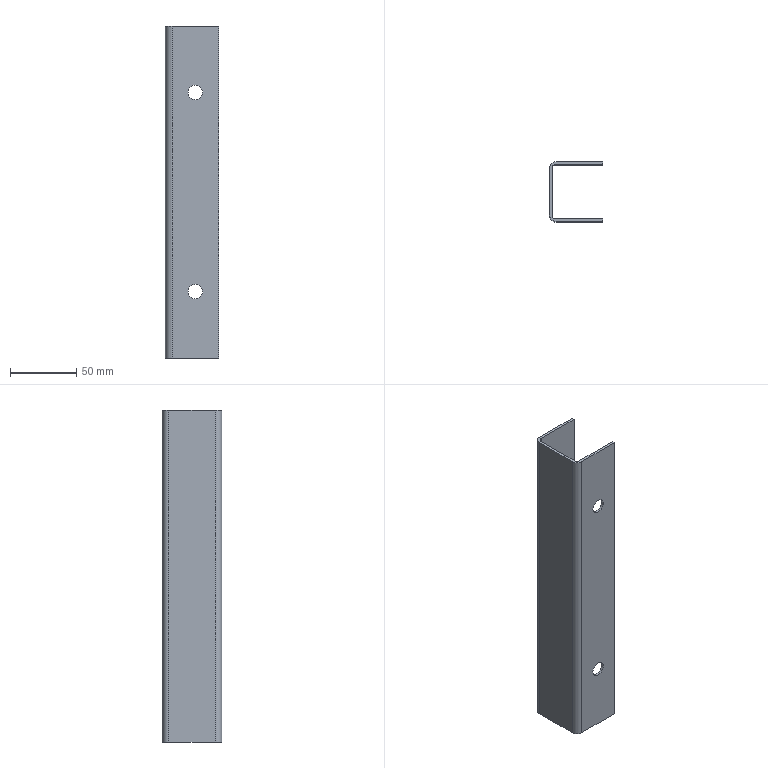Part | STEP file | Channel 50x30x2x3-250 GOST 8278-83 | 1 solid | 18 faces | box 40 x 45 x 250 mm | volume 58023 mm3 | plane 10 | cylinder 8 | commonest cylinder face diameters 11 x4 6 x2 10 x2
STEP:
#1=CARTESIAN_POINT('',(0.,0.,0.));
#2=DIRECTION('',(0.,0.,1.));
#3=DIRECTION('',(1.,0.,0.));
#4=AXIS2_PLACEMENT_3D('',#1,#2,#3);
#5=CARTESIAN_POINT('',(18.8,-18.,200.));
#6=VERTEX_POINT('',#5);
#7=CARTESIAN_POINT('',(13.3,-18.,200.));
#8=DIRECTION('',(0.,-1.,0.));
#9=DIRECTION('',(-1.,0.,0.));
#10=AXIS2_PLACEMENT_3D('',#7,#8,#9);
#11=CIRCLE('',#10,5.5);
#12=CARTESIAN_POINT('',(13.3,25.,200.));
#13=DIRECTION('',(0.,1.,0.));
#14=DIRECTION('',(-1.,0.,0.));
#15=AXIS2_PLACEMENT_3D('',#12,#13,#14);
#16=CYLINDRICAL_SURFACE('',#15,5.5);
#17=CARTESIAN_POINT('',(12.566,-43.));
#18=DIRECTION('',(-1.,0.));
#19=VECTOR('',#18,1.);
#20=LINE('',#17,#19);
#21=(GEOMETRIC_REPRESENTATION_CONTEXT(2)PARAMETRIC_REPRESENTATION_CONTEXT()REPRESENTATION_CONTEXT('',''));
#22=DEFINITIONAL_REPRESENTATION('',(#20),#21);
#23=PCURVE('',#16,#22);
#24=CARTESIAN_POINT('',(-4.2,-18.,0.));
#25=DIRECTION('',(0.,1.,0.));
#26=DIRECTION('',(0.,0.,1.));
#27=AXIS2_PLACEMENT_3D('',#24,#25,#26);
#28=PLANE('',#27);
#29=CARTESIAN_POINT('',(200.,12.));
#30=CARTESIAN_POINT('',(190.474,12.));
#31=CARTESIAN_POINT('',(195.237,20.25));
#32=CARTESIAN_POINT('',(200.,28.5));
#33=CARTESIAN_POINT('',(204.763,20.25));
#34=CARTESIAN_POINT('',(209.526,12.));
#35=CARTESIAN_POINT('',(200.,12.));
#36=(BOUNDED_CURVE()B_SPLINE_CURVE(2,(#29,#30,#31,#32,#33,#34,#35),.UNSPECIFIED.,.T.,.F.)B_SPLINE_CURVE_WITH_KNOTS((1,2,2,2,2,1),(-2.094,0.,2.094,4.189,6.283,8.378),.UNSPECIFIED.)CURVE()GEOMETRIC_REPRESENTATION_ITEM()RATIONAL_B_SPLINE_CURVE((1.,0.5,1.,0.5,1.,0.5,1.))REPRESENTATION_ITEM(''));
#37=(GEOMETRIC_REPRESENTATION_CONTEXT(2)PARAMETRIC_REPRESENTATION_CONTEXT()REPRESENTATION_CONTEXT('',''));
#38=DEFINITIONAL_REPRESENTATION('',(#36),#37);
#39=PCURVE('',#28,#38);
#40=SURFACE_CURVE('',#11,(#23,#39),.PCURVE_S1.);
#41=EDGE_CURVE('',#6,#6,#40,.T.);
#42=ORIENTED_EDGE('',*,*,#41,.T.);
#43=CARTESIAN_POINT('',(18.8,-20.,200.));
#44=VERTEX_POINT('',#43);
#45=CARTESIAN_POINT('',(18.8,-20.,200.));
#46=CARTESIAN_POINT('',(18.8,-18.,200.));
#47=B_SPLINE_CURVE_WITH_KNOTS('',1,(#45,#46),.UNSPECIFIED.,.F.,.F.,(2,2),(-45.,-43.),.PIECEWISE_BEZIER_KNOTS.);
#48=CARTESIAN_POINT('',(3.142,0.));
#49=DIRECTION('',(0.,1.));
#50=VECTOR('',#49,1.);
#51=LINE('',#48,#50);
#52=(GEOMETRIC_REPRESENTATION_CONTEXT(2)PARAMETRIC_REPRESENTATION_CONTEXT()REPRESENTATION_CONTEXT('',''));
#53=DEFINITIONAL_REPRESENTATION('',(#51),#52);
#54=PCURVE('',#16,#53);
#55=CARTESIAN_POINT('',(9.425,0.));
#56=DIRECTION('',(0.,1.));
#57=VECTOR('',#56,1.);
#58=LINE('',#55,#57);
#59=(GEOMETRIC_REPRESENTATION_CONTEXT(2)PARAMETRIC_REPRESENTATION_CONTEXT()REPRESENTATION_CONTEXT('',''));
#60=DEFINITIONAL_REPRESENTATION('',(#58),#59);
#61=PCURVE('',#16,#60);
#62=SEAM_CURVE('',#47,(#54,#61),.PCURVE_S1.);
#63=EDGE_CURVE('',#44,#6,#62,.T.);
#64=ORIENTED_EDGE('',*,*,#63,.F.);
#65=CARTESIAN_POINT('',(13.3,-20.,200.));
#66=DIRECTION('',(0.,1.,0.));
#67=DIRECTION('',(-1.,0.,0.));
#68=AXIS2_PLACEMENT_3D('',#65,#66,#67);
#69=CIRCLE('',#68,5.5);
#70=CARTESIAN_POINT('',(0.,-45.));
#71=DIRECTION('',(1.,0.));
#72=VECTOR('',#71,1.);
#73=LINE('',#70,#72);
#74=(GEOMETRIC_REPRESENTATION_CONTEXT(2)PARAMETRIC_REPRESENTATION_CONTEXT()REPRESENTATION_CONTEXT('',''));
#75=DEFINITIONAL_REPRESENTATION('',(#73),#74);
#76=PCURVE('',#16,#75);
#77=CARTESIAN_POINT('',(30.8,-20.,0.));
#78=DIRECTION('',(0.,-1.,0.));
#79=DIRECTION('',(0.,0.,-1.));
#80=AXIS2_PLACEMENT_3D('',#77,#78,#79);
#81=PLANE('',#80);
#82=CARTESIAN_POINT('',(-200.,-23.));
#83=CARTESIAN_POINT('',(-209.526,-23.));
#84=CARTESIAN_POINT('',(-204.763,-14.75));
#85=CARTESIAN_POINT('',(-200.,-6.5));
#86=CARTESIAN_POINT('',(-195.237,-14.75));
#87=CARTESIAN_POINT('',(-190.474,-23.));
#88=CARTESIAN_POINT('',(-200.,-23.));
#89=(BOUNDED_CURVE()B_SPLINE_CURVE(2,(#82,#83,#84,#85,#86,#87,#88),.UNSPECIFIED.,.T.,.F.)B_SPLINE_CURVE_WITH_KNOTS((1,2,2,2,2,1),(-2.094,0.,2.094,4.189,6.283,8.378),.UNSPECIFIED.)CURVE()GEOMETRIC_REPRESENTATION_ITEM()RATIONAL_B_SPLINE_CURVE((1.,0.5,1.,0.5,1.,0.5,1.))REPRESENTATION_ITEM(''));
#90=(GEOMETRIC_REPRESENTATION_CONTEXT(2)PARAMETRIC_REPRESENTATION_CONTEXT()REPRESENTATION_CONTEXT('',''));
#91=DEFINITIONAL_REPRESENTATION('',(#89),#90);
#92=PCURVE('',#81,#91);
#93=SURFACE_CURVE('',#69,(#76,#92),.PCURVE_S1.);
#94=EDGE_CURVE('',#44,#44,#93,.T.);
#95=ORIENTED_EDGE('',*,*,#94,.T.);
#96=ORIENTED_EDGE('',*,*,#63,.T.);
#97=EDGE_LOOP('',(#42,#64,#95,#96));
#98=FACE_BOUND('',#97,.F.);
#99=ADVANCED_FACE('',(#98),#16,.F.);
#100=CARTESIAN_POINT('',(18.8,25.,200.));
#101=VERTEX_POINT('',#100);
#102=CARTESIAN_POINT('',(13.3,25.,200.));
#103=DIRECTION('',(0.,-1.,0.));
#104=DIRECTION('',(-1.,0.,0.));
#105=AXIS2_PLACEMENT_3D('',#102,#103,#104);
#106=CIRCLE('',#105,5.5);
#107=CARTESIAN_POINT('',(13.3,25.,200.));
#108=DIRECTION('',(0.,1.,0.));
#109=DIRECTION('',(-1.,0.,0.));
#110=AXIS2_PLACEMENT_3D('',#107,#108,#109);
#111=CYLINDRICAL_SURFACE('',#110,5.5);
#112=CARTESIAN_POINT('',(12.566,0.));
#113=DIRECTION('',(-1.,0.));
#114=VECTOR('',#113,1.);
#115=LINE('',#112,#114);
#116=(GEOMETRIC_REPRESENTATION_CONTEXT(2)PARAMETRIC_REPRESENTATION_CONTEXT()REPRESENTATION_CONTEXT('',''));
#117=DEFINITIONAL_REPRESENTATION('',(#115),#116);
#118=PCURVE('',#111,#117);
#119=CARTESIAN_POINT('',(-4.2,25.,0.));
#120=DIRECTION('',(0.,1.,0.));
#121=DIRECTION('',(0.,0.,1.));
#122=AXIS2_PLACEMENT_3D('',#119,#120,#121);
#123=PLANE('',#122);
#124=CARTESIAN_POINT('',(200.,12.));
#125=CARTESIAN_POINT('',(190.474,12.));
#126=CARTESIAN_POINT('',(195.237,20.25));
#127=CARTESIAN_POINT('',(200.,28.5));
#128=CARTESIAN_POINT('',(204.763,20.25));
#129=CARTESIAN_POINT('',(209.526,12.));
#130=CARTESIAN_POINT('',(200.,12.));
#131=(BOUNDED_CURVE()B_SPLINE_CURVE(2,(#124,#125,#126,#127,#128,#129,#130),.UNSPECIFIED.,.T.,.F.)B_SPLINE_CURVE_WITH_KNOTS((1,2,2,2,2,1),(-2.094,0.,2.094,4.189,6.283,8.378),.UNSPECIFIED.)CURVE()GEOMETRIC_REPRESENTATION_ITEM()RATIONAL_B_SPLINE_CURVE((1.,0.5,1.,0.5,1.,0.5,1.))REPRESENTATION_ITEM(''));
#132=(GEOMETRIC_REPRESENTATION_CONTEXT(2)PARAMETRIC_REPRESENTATION_CONTEXT()REPRESENTATION_CONTEXT('',''));
#133=DEFINITIONAL_REPRESENTATION('',(#131),#132);
#134=PCURVE('',#123,#133);
#135=SURFACE_CURVE('',#106,(#118,#134),.PCURVE_S1.);
#136=EDGE_CURVE('',#101,#101,#135,.T.);
#137=ORIENTED_EDGE('',*,*,#136,.T.);
#138=CARTESIAN_POINT('',(18.8,23.,200.));
#139=VERTEX_POINT('',#138);
#140=CARTESIAN_POINT('',(18.8,23.,200.));
#141=CARTESIAN_POINT('',(18.8,25.,200.));
#142=B_SPLINE_CURVE_WITH_KNOTS('',1,(#140,#141),.UNSPECIFIED.,.F.,.F.,(2,2),(-2.,0.),.PIECEWISE_BEZIER_KNOTS.);
#143=CARTESIAN_POINT('',(3.142,0.));
#144=DIRECTION('',(0.,1.));
#145=VECTOR('',#144,1.);
#146=LINE('',#143,#145);
#147=(GEOMETRIC_REPRESENTATION_CONTEXT(2)PARAMETRIC_REPRESENTATION_CONTEXT()REPRESENTATION_CONTEXT('',''));
#148=DEFINITIONAL_REPRESENTATION('',(#146),#147);
#149=PCURVE('',#111,#148);
#150=CARTESIAN_POINT('',(9.425,0.));
#151=DIRECTION('',(0.,1.));
#152=VECTOR('',#151,1.);
#153=LINE('',#150,#152);
#154=(GEOMETRIC_REPRESENTATION_CONTEXT(2)PARAMETRIC_REPRESENTATION_CONTEXT()REPRESENTATION_CONTEXT('',''));
#155=DEFINITIONAL_REPRESENTATION('',(#153),#154);
#156=PCURVE('',#111,#155);
#157=SEAM_CURVE('',#142,(#149,#156),.PCURVE_S1.);
#158=EDGE_CURVE('',#139,#101,#157,.T.);
#159=ORIENTED_EDGE('',*,*,#158,.F.);
#160=CARTESIAN_POINT('',(13.3,23.,200.));
#161=DIRECTION('',(0.,1.,0.));
#162=DIRECTION('',(-1.,0.,0.));
#163=AXIS2_PLACEMENT_3D('',#160,#161,#162);
#164=CIRCLE('',#163,5.5);
#165=CARTESIAN_POINT('',(0.,-2.));
#166=DIRECTION('',(1.,0.));
#167=VECTOR('',#166,1.);
#168=LINE('',#165,#167);
#169=(GEOMETRIC_REPRESENTATION_CONTEXT(2)PARAMETRIC_REPRESENTATION_CONTEXT()REPRESENTATION_CONTEXT('',''));
#170=DEFINITIONAL_REPRESENTATION('',(#168),#169);
#171=PCURVE('',#111,#170);
#172=CARTESIAN_POINT('',(30.8,23.,0.));
#173=DIRECTION('',(0.,-1.,0.));
#174=DIRECTION('',(0.,0.,-1.));
#175=AXIS2_PLACEMENT_3D('',#172,#173,#174);
#176=PLANE('',#175);
#177=CARTESIAN_POINT('',(-200.,-23.));
#178=CARTESIAN_POINT('',(-209.526,-23.));
#179=CARTESIAN_POINT('',(-204.763,-14.75));
#180=CARTESIAN_POINT('',(-200.,-6.5));
#181=CARTESIAN_POINT('',(-195.237,-14.75));
#182=CARTESIAN_POINT('',(-190.474,-23.));
#183=CARTESIAN_POINT('',(-200.,-23.));
#184=(BOUNDED_CURVE()B_SPLINE_CURVE(2,(#177,#178,#179,#180,#181,#182,#183),.UNSPECIFIED.,.T.,.F.)B_SPLINE_CURVE_WITH_KNOTS((1,2,2,2,2,1),(-2.094,0.,2.094,4.189,6.283,8.378),.UNSPECIFIED.)CURVE()GEOMETRIC_REPRESENTATION_ITEM()RATIONAL_B_SPLINE_CURVE((1.,0.5,1.,0.5,1.,0.5,1.))REPRESENTATION_ITEM(''));
#185=(GEOMETRIC_REPRESENTATION_CONTEXT(2)PARAMETRIC_REPRESENTATION_CONTEXT()REPRESENTATION_CONTEXT('',''));
#186=DEFINITIONAL_REPRESENTATION('',(#184),#185);
#187=PCURVE('',#176,#186);
#188=SURFACE_CURVE('',#164,(#171,#187),.PCURVE_S1.);
#189=EDGE_CURVE('',#139,#139,#188,.T.);
#190=ORIENTED_EDGE('',*,*,#189,.T.);
#191=ORIENTED_EDGE('',*,*,#158,.T.);
#192=EDGE_LOOP('',(#137,#159,#190,#191));
#193=FACE_BOUND('',#192,.F.);
#194=ADVANCED_FACE('',(#193),#111,.F.);
#195=CARTESIAN_POINT('',(18.8,-18.,50.));
#196=VERTEX_POINT('',#195);
#197=CARTESIAN_POINT('',(13.3,-18.,50.));
#198=DIRECTION('',(0.,-1.,0.));
#199=DIRECTION('',(-1.,0.,0.));
#200=AXIS2_PLACEMENT_3D('',#197,#198,#199);
#201=CIRCLE('',#200,5.5);
#202=CARTESIAN_POINT('',(13.3,25.,50.));
#203=DIRECTION('',(0.,1.,0.));
#204=DIRECTION('',(-1.,0.,0.));
#205=AXIS2_PLACEMENT_3D('',#202,#203,#204);
#206=CYLINDRICAL_SURFACE('',#205,5.5);
#207=CARTESIAN_POINT('',(12.566,-43.));
#208=DIRECTION('',(-1.,0.));
#209=VECTOR('',#208,1.);
#210=LINE('',#207,#209);
#211=(GEOMETRIC_REPRESENTATION_CONTEXT(2)PARAMETRIC_REPRESENTATION_CONTEXT()REPRESENTATION_CONTEXT('',''));
#212=DEFINITIONAL_REPRESENTATION('',(#210),#211);
#213=PCURVE('',#206,#212);
#214=CARTESIAN_POINT('',(50.,12.));
#215=CARTESIAN_POINT('',(40.474,12.));
#216=CARTESIAN_POINT('',(45.237,20.25));
#217=CARTESIAN_POINT('',(50.,28.5));
#218=CARTESIAN_POINT('',(54.763,20.25));
#219=CARTESIAN_POINT('',(59.526,12.));
#220=CARTESIAN_POINT('',(50.,12.));
#221=(BOUNDED_CURVE()B_SPLINE_CURVE(2,(#214,#215,#216,#217,#218,#219,#220),.UNSPECIFIED.,.T.,.F.)B_SPLINE_CURVE_WITH_KNOTS((1,2,2,2,2,1),(-2.094,0.,2.094,4.189,6.283,8.378),.UNSPECIFIED.)CURVE()GEOMETRIC_REPRESENTATION_ITEM()RATIONAL_B_SPLINE_CURVE((1.,0.5,1.,0.5,1.,0.5,1.))REPRESENTATION_ITEM(''));
#222=(GEOMETRIC_REPRESENTATION_CONTEXT(2)PARAMETRIC_REPRESENTATION_CONTEXT()REPRESENTATION_CONTEXT('',''));
#223=DEFINITIONAL_REPRESENTATION('',(#221),#222);
#224=PCURVE('',#28,#223);
#225=SURFACE_CURVE('',#201,(#213,#224),.PCURVE_S1.);
#226=EDGE_CURVE('',#196,#196,#225,.T.);
#227=ORIENTED_EDGE('',*,*,#226,.T.);
#228=CARTESIAN_POINT('',(18.8,-20.,50.));
#229=VERTEX_POINT('',#228);
#230=CARTESIAN_POINT('',(18.8,-20.,50.));
#231=CARTESIAN_POINT('',(18.8,-18.,50.));
#232=B_SPLINE_CURVE_WITH_KNOTS('',1,(#230,#231),.UNSPECIFIED.,.F.,.F.,(2,2),(-45.,-43.),.PIECEWISE_BEZIER_KNOTS.);
#233=CARTESIAN_POINT('',(3.142,0.));
#234=DIRECTION('',(0.,1.));
#235=VECTOR('',#234,1.);
#236=LINE('',#233,#235);
#237=(GEOMETRIC_REPRESENTATION_CONTEXT(2)PARAMETRIC_REPRESENTATION_CONTEXT()REPRESENTATION_CONTEXT('',''));
#238=DEFINITIONAL_REPRESENTATION('',(#236),#237);
#239=PCURVE('',#206,#238);
#240=CARTESIAN_POINT('',(9.425,0.));
#241=DIRECTION('',(0.,1.));
#242=VECTOR('',#241,1.);
#243=LINE('',#240,#242);
#244=(GEOMETRIC_REPRESENTATION_CONTEXT(2)PARAMETRIC_REPRESENTATION_CONTEXT()REPRESENTATION_CONTEXT('',''));
#245=DEFINITIONAL_REPRESENTATION('',(#243),#244);
#246=PCURVE('',#206,#245);
#247=SEAM_CURVE('',#232,(#239,#246),.PCURVE_S1.);
#248=EDGE_CURVE('',#229,#196,#247,.T.);
#249=ORIENTED_EDGE('',*,*,#248,.F.);
#250=CARTESIAN_POINT('',(13.3,-20.,50.));
#251=DIRECTION('',(0.,1.,0.));
#252=DIRECTION('',(-1.,0.,0.));
#253=AXIS2_PLACEMENT_3D('',#250,#251,#252);
#254=CIRCLE('',#253,5.5);
#255=CARTESIAN_POINT('',(0.,-45.));
#256=DIRECTION('',(1.,0.));
#257=VECTOR('',#256,1.);
#258=LINE('',#255,#257);
#259=(GEOMETRIC_REPRESENTATION_CONTEXT(2)PARAMETRIC_REPRESENTATION_CONTEXT()REPRESENTATION_CONTEXT('',''));
#260=DEFINITIONAL_REPRESENTATION('',(#258),#259);
#261=PCURVE('',#206,#260);
#262=CARTESIAN_POINT('',(-50.,-23.));
#263=CARTESIAN_POINT('',(-59.526,-23.));
#264=CARTESIAN_POINT('',(-54.763,-14.75));
#265=CARTESIAN_POINT('',(-50.,-6.5));
#266=CARTESIAN_POINT('',(-45.237,-14.75));
#267=CARTESIAN_POINT('',(-40.474,-23.));
#268=CARTESIAN_POINT('',(-50.,-23.));
#269=(BOUNDED_CURVE()B_SPLINE_CURVE(2,(#262,#263,#264,#265,#266,#267,#268),.UNSPECIFIED.,.T.,.F.)B_SPLINE_CURVE_WITH_KNOTS((1,2,2,2,2,1),(-2.094,0.,2.094,4.189,6.283,8.378),.UNSPECIFIED.)CURVE()GEOMETRIC_REPRESENTATION_ITEM()RATIONAL_B_SPLINE_CURVE((1.,0.5,1.,0.5,1.,0.5,1.))REPRESENTATION_ITEM(''));
#270=(GEOMETRIC_REPRESENTATION_CONTEXT(2)PARAMETRIC_REPRESENTATION_CONTEXT()REPRESENTATION_CONTEXT('',''));
#271=DEFINITIONAL_REPRESENTATION('',(#269),#270);
#272=PCURVE('',#81,#271);
#273=SURFACE_CURVE('',#254,(#261,#272),.PCURVE_S1.);
#274=EDGE_CURVE('',#229,#229,#273,.T.);
#275=ORIENTED_EDGE('',*,*,#274,.T.);
#276=ORIENTED_EDGE('',*,*,#248,.T.);
#277=EDGE_LOOP('',(#227,#249,#275,#276));
#278=FACE_BOUND('',#277,.F.);
#279=ADVANCED_FACE('',(#278),#206,.F.);
#280=CARTESIAN_POINT('',(18.8,25.,50.));
#281=VERTEX_POINT('',#280);
#282=CARTESIAN_POINT('',(13.3,25.,50.));
#283=DIRECTION('',(0.,-1.,0.));
#284=DIRECTION('',(-1.,0.,0.));
#285=AXIS2_PLACEMENT_3D('',#282,#283,#284);
#286=CIRCLE('',#285,5.5);
#287=CARTESIAN_POINT('',(13.3,25.,50.));
#288=DIRECTION('',(0.,1.,0.));
#289=DIRECTION('',(-1.,0.,0.));
#290=AXIS2_PLACEMENT_3D('',#287,#288,#289);
#291=CYLINDRICAL_SURFACE('',#290,5.5);
#292=CARTESIAN_POINT('',(12.566,0.));
#293=DIRECTION('',(-1.,0.));
#294=VECTOR('',#293,1.);
#295=LINE('',#292,#294);
#296=(GEOMETRIC_REPRESENTATION_CONTEXT(2)PARAMETRIC_REPRESENTATION_CONTEXT()REPRESENTATION_CONTEXT('',''));
#297=DEFINITIONAL_REPRESENTATION('',(#295),#296);
#298=PCURVE('',#291,#297);
#299=CARTESIAN_POINT('',(50.,12.));
#300=CARTESIAN_POINT('',(40.474,12.));
#301=CARTESIAN_POINT('',(45.237,20.25));
#302=CARTESIAN_POINT('',(50.,28.5));
#303=CARTESIAN_POINT('',(54.763,20.25));
#304=CARTESIAN_POINT('',(59.526,12.));
#305=CARTESIAN_POINT('',(50.,12.));
#306=(BOUNDED_CURVE()B_SPLINE_CURVE(2,(#299,#300,#301,#302,#303,#304,#305),.UNSPECIFIED.,.T.,.F.)B_SPLINE_CURVE_WITH_KNOTS((1,2,2,2,2,1),(-2.094,0.,2.094,4.189,6.283,8.378),.UNSPECIFIED.)CURVE()GEOMETRIC_REPRESENTATION_ITEM()RATIONAL_B_SPLINE_CURVE((1.,0.5,1.,0.5,1.,0.5,1.))REPRESENTATION_ITEM(''));
#307=(GEOMETRIC_REPRESENTATION_CONTEXT(2)PARAMETRIC_REPRESENTATION_CONTEXT()REPRESENTATION_CONTEXT('',''));
#308=DEFINITIONAL_REPRESENTATION('',(#306),#307);
#309=PCURVE('',#123,#308);
#310=SURFACE_CURVE('',#286,(#298,#309),.PCURVE_S1.);
#311=EDGE_CURVE('',#281,#281,#310,.T.);
#312=ORIENTED_EDGE('',*,*,#311,.T.);
#313=CARTESIAN_POINT('',(18.8,23.,50.));
#314=VERTEX_POINT('',#313);
#315=CARTESIAN_POINT('',(18.8,23.,50.));
#316=CARTESIAN_POINT('',(18.8,25.,50.));
#317=B_SPLINE_CURVE_WITH_KNOTS('',1,(#315,#316),.UNSPECIFIED.,.F.,.F.,(2,2),(-2.,0.),.PIECEWISE_BEZIER_KNOTS.);
#318=CARTESIAN_POINT('',(3.142,0.));
#319=DIRECTION('',(0.,1.));
#320=VECTOR('',#319,1.);
#321=LINE('',#318,#320);
#322=(GEOMETRIC_REPRESENTATION_CONTEXT(2)PARAMETRIC_REPRESENTATION_CONTEXT()REPRESENTATION_CONTEXT('',''));
#323=DEFINITIONAL_REPRESENTATION('',(#321),#322);
#324=PCURVE('',#291,#323);
#325=CARTESIAN_POINT('',(9.425,0.));
#326=DIRECTION('',(0.,1.));
#327=VECTOR('',#326,1.);
#328=LINE('',#325,#327);
#329=(GEOMETRIC_REPRESENTATION_CONTEXT(2)PARAMETRIC_REPRESENTATION_CONTEXT()REPRESENTATION_CONTEXT('',''));
#330=DEFINITIONAL_REPRESENTATION('',(#328),#329);
#331=PCURVE('',#291,#330);
#332=SEAM_CURVE('',#317,(#324,#331),.PCURVE_S1.);
#333=EDGE_CURVE('',#314,#281,#332,.T.);
#334=ORIENTED_EDGE('',*,*,#333,.F.);
#335=CARTESIAN_POINT('',(13.3,23.,50.));
#336=DIRECTION('',(0.,1.,0.));
#337=DIRECTION('',(-1.,0.,0.));
#338=AXIS2_PLACEMENT_3D('',#335,#336,#337);
#339=CIRCLE('',#338,5.5);
#340=CARTESIAN_POINT('',(0.,-2.));
#341=DIRECTION('',(1.,0.));
#342=VECTOR('',#341,1.);
#343=LINE('',#340,#342);
#344=(GEOMETRIC_REPRESENTATION_CONTEXT(2)PARAMETRIC_REPRESENTATION_CONTEXT()REPRESENTATION_CONTEXT('',''));
#345=DEFINITIONAL_REPRESENTATION('',(#343),#344);
#346=PCURVE('',#291,#345);
#347=CARTESIAN_POINT('',(-50.,-23.));
#348=CARTESIAN_POINT('',(-59.526,-23.));
#349=CARTESIAN_POINT('',(-54.763,-14.75));
#350=CARTESIAN_POINT('',(-50.,-6.5));
#351=CARTESIAN_POINT('',(-45.237,-14.75));
#352=CARTESIAN_POINT('',(-40.474,-23.));
#353=CARTESIAN_POINT('',(-50.,-23.));
#354=(BOUNDED_CURVE()B_SPLINE_CURVE(2,(#347,#348,#349,#350,#351,#352,#353),.UNSPECIFIED.,.T.,.F.)B_SPLINE_CURVE_WITH_KNOTS((1,2,2,2,2,1),(-2.094,0.,2.094,4.189,6.283,8.378),.UNSPECIFIED.)CURVE()GEOMETRIC_REPRESENTATION_ITEM()RATIONAL_B_SPLINE_CURVE((1.,0.5,1.,0.5,1.,0.5,1.))REPRESENTATION_ITEM(''));
#355=(GEOMETRIC_REPRESENTATION_CONTEXT(2)PARAMETRIC_REPRESENTATION_CONTEXT()REPRESENTATION_CONTEXT('',''));
#356=DEFINITIONAL_REPRESENTATION('',(#354),#355);
#357=PCURVE('',#176,#356);
#358=SURFACE_CURVE('',#339,(#346,#357),.PCURVE_S1.);
#359=EDGE_CURVE('',#314,#314,#358,.T.);
#360=ORIENTED_EDGE('',*,*,#359,.T.);
#361=ORIENTED_EDGE('',*,*,#333,.T.);
#362=EDGE_LOOP('',(#312,#334,#360,#361));
#363=FACE_BOUND('',#362,.F.);
#364=ADVANCED_FACE('',(#363),#291,.F.);
#365=CARTESIAN_POINT('',(30.8,-20.,250.));
#366=VERTEX_POINT('',#365);
#367=CARTESIAN_POINT('',(-4.2,-20.,250.));
#368=VERTEX_POINT('',#367);
#369=CARTESIAN_POINT('',(20.8,-20.,250.));
#370=DIRECTION('',(-1.,0.,0.));
#371=VECTOR('',#370,1.);
#372=LINE('',#369,#371);
#373=CARTESIAN_POINT('',(-250.,-10.));
#374=DIRECTION('',(0.,-1.));
#375=VECTOR('',#374,1.);
#376=LINE('',#373,#375);
#377=(GEOMETRIC_REPRESENTATION_CONTEXT(2)PARAMETRIC_REPRESENTATION_CONTEXT()REPRESENTATION_CONTEXT('',''));
#378=DEFINITIONAL_REPRESENTATION('',(#376),#377);
#379=PCURVE('',#81,#378);
#380=CARTESIAN_POINT('',(10.8,2.5,250.));
#381=DIRECTION('',(0.,0.,1.));
#382=DIRECTION('',(1.,0.,0.));
#383=AXIS2_PLACEMENT_3D('',#380,#381,#382);
#384=PLANE('',#383);
#385=CARTESIAN_POINT('',(10.,-22.5));
#386=DIRECTION('',(-1.,0.));
#387=VECTOR('',#386,1.);
#388=LINE('',#385,#387);
#389=(GEOMETRIC_REPRESENTATION_CONTEXT(2)PARAMETRIC_REPRESENTATION_CONTEXT()REPRESENTATION_CONTEXT('',''));
#390=DEFINITIONAL_REPRESENTATION('',(#388),#389);
#391=PCURVE('',#384,#390);
#392=SURFACE_CURVE('',#372,(#379,#391),.PCURVE_S1.);
#393=EDGE_CURVE('',#366,#368,#392,.T.);
#394=ORIENTED_EDGE('',*,*,#393,.T.);
#395=CARTESIAN_POINT('',(-4.2,-20.,0.));
#396=VERTEX_POINT('',#395);
#397=CARTESIAN_POINT('',(-4.2,-20.,0.));
#398=DIRECTION('',(0.,0.,1.));
#399=VECTOR('',#398,1.);
#400=LINE('',#397,#399);
#401=CARTESIAN_POINT('',(0.,-35.));
#402=DIRECTION('',(-1.,0.));
#403=VECTOR('',#402,1.);
#404=LINE('',#401,#403);
#405=(GEOMETRIC_REPRESENTATION_CONTEXT(2)PARAMETRIC_REPRESENTATION_CONTEXT()REPRESENTATION_CONTEXT('',''));
#406=DEFINITIONAL_REPRESENTATION('',(#404),#405);
#407=PCURVE('',#81,#406);
#408=CARTESIAN_POINT('',(-4.2,-15.,0.));
#409=DIRECTION('',(0.,0.,1.));
#410=DIRECTION('',(1.,0.,0.));
#411=AXIS2_PLACEMENT_3D('',#408,#409,#410);
#412=CYLINDRICAL_SURFACE('',#411,5.);
#413=CARTESIAN_POINT('',(4.712,0.));
#414=DIRECTION('',(0.,1.));
#415=VECTOR('',#414,1.);
#416=LINE('',#413,#415);
#417=(GEOMETRIC_REPRESENTATION_CONTEXT(2)PARAMETRIC_REPRESENTATION_CONTEXT()REPRESENTATION_CONTEXT('',''));
#418=DEFINITIONAL_REPRESENTATION('',(#416),#417);
#419=PCURVE('',#412,#418);
#420=SURFACE_CURVE('',#400,(#407,#419),.PCURVE_S1.);
#421=EDGE_CURVE('',#396,#368,#420,.T.);
#422=ORIENTED_EDGE('',*,*,#421,.F.);
#423=CARTESIAN_POINT('',(30.8,-20.,0.));
#424=VERTEX_POINT('',#423);
#425=CARTESIAN_POINT('',(20.8,-20.,0.));
#426=DIRECTION('',(-1.,0.,0.));
#427=VECTOR('',#426,1.);
#428=LINE('',#425,#427);
#429=CARTESIAN_POINT('',(0.,-10.));
#430=DIRECTION('',(0.,-1.));
#431=VECTOR('',#430,1.);
#432=LINE('',#429,#431);
#433=(GEOMETRIC_REPRESENTATION_CONTEXT(2)PARAMETRIC_REPRESENTATION_CONTEXT()REPRESENTATION_CONTEXT('',''));
#434=DEFINITIONAL_REPRESENTATION('',(#432),#433);
#435=PCURVE('',#81,#434);
#436=CARTESIAN_POINT('',(10.8,2.5,0.));
#437=DIRECTION('',(0.,0.,1.));
#438=DIRECTION('',(1.,0.,0.));
#439=AXIS2_PLACEMENT_3D('',#436,#437,#438);
#440=PLANE('',#439);
#441=CARTESIAN_POINT('',(10.,-22.5));
#442=DIRECTION('',(-1.,0.));
#443=VECTOR('',#442,1.);
#444=LINE('',#441,#443);
#445=(GEOMETRIC_REPRESENTATION_CONTEXT(2)PARAMETRIC_REPRESENTATION_CONTEXT()REPRESENTATION_CONTEXT('',''));
#446=DEFINITIONAL_REPRESENTATION('',(#444),#445);
#447=PCURVE('',#440,#446);
#448=SURFACE_CURVE('',#428,(#435,#447),.PCURVE_S1.);
#449=EDGE_CURVE('',#424,#396,#448,.T.);
#450=ORIENTED_EDGE('',*,*,#449,.F.);
#451=CARTESIAN_POINT('',(30.8,-20.,0.));
#452=DIRECTION('',(0.,0.,1.));
#453=VECTOR('',#452,1.);
#454=LINE('',#451,#453);
#455=CARTESIAN_POINT('',(0.,0.));
#456=DIRECTION('',(-1.,0.));
#457=VECTOR('',#456,1.);
#458=LINE('',#455,#457);
#459=(GEOMETRIC_REPRESENTATION_CONTEXT(2)PARAMETRIC_REPRESENTATION_CONTEXT()REPRESENTATION_CONTEXT('',''));
#460=DEFINITIONAL_REPRESENTATION('',(#458),#459);
#461=PCURVE('',#81,#460);
#462=CARTESIAN_POINT('',(30.8,-18.,0.));
#463=DIRECTION('',(1.,0.,0.));
#464=DIRECTION('',(0.,0.,-1.));
#465=AXIS2_PLACEMENT_3D('',#462,#463,#464);
#466=PLANE('',#465);
#467=CARTESIAN_POINT('',(0.,-2.));
#468=DIRECTION('',(-1.,0.));
#469=VECTOR('',#468,1.);
#470=LINE('',#467,#469);
#471=(GEOMETRIC_REPRESENTATION_CONTEXT(2)PARAMETRIC_REPRESENTATION_CONTEXT()REPRESENTATION_CONTEXT('',''));
#472=DEFINITIONAL_REPRESENTATION('',(#470),#471);
#473=PCURVE('',#466,#472);
#474=SURFACE_CURVE('',#454,(#461,#473),.PCURVE_S1.);
#475=EDGE_CURVE('',#424,#366,#474,.T.);
#476=ORIENTED_EDGE('',*,*,#475,.T.);
#477=EDGE_LOOP('',(#394,#422,#450,#476));
#478=FACE_BOUND('',#477,.T.);
#479=ORIENTED_EDGE('',*,*,#94,.T.);
#480=EDGE_LOOP('',(#479));
#481=FACE_BOUND('',#480,.T.);
#482=ORIENTED_EDGE('',*,*,#274,.T.);
#483=EDGE_LOOP('',(#482));
#484=FACE_BOUND('',#483,.T.);
#485=ADVANCED_FACE('',(#478,#481,#484),#81,.T.);
#486=CARTESIAN_POINT('',(-9.2,-15.,250.));
#487=VERTEX_POINT('',#486);
#488=CARTESIAN_POINT('',(-4.2,-15.,250.));
#489=DIRECTION('',(0.,0.,-1.));
#490=DIRECTION('',(1.,0.,0.));
#491=AXIS2_PLACEMENT_3D('',#488,#489,#490);
#492=CIRCLE('',#491,5.);
#493=CARTESIAN_POINT('',(6.283,250.));
#494=DIRECTION('',(-1.,0.));
#495=VECTOR('',#494,1.);
#496=LINE('',#493,#495);
#497=(GEOMETRIC_REPRESENTATION_CONTEXT(2)PARAMETRIC_REPRESENTATION_CONTEXT()REPRESENTATION_CONTEXT('',''));
#498=DEFINITIONAL_REPRESENTATION('',(#496),#497);
#499=PCURVE('',#412,#498);
#500=CARTESIAN_POINT('',(-10.,-17.5));
#501=CARTESIAN_POINT('',(-10.,-26.16));
#502=CARTESIAN_POINT('',(-17.5,-21.83));
#503=CARTESIAN_POINT('',(-25.,-17.5));
#504=CARTESIAN_POINT('',(-17.5,-13.17));
#505=CARTESIAN_POINT('',(-10.,-8.84));
#506=CARTESIAN_POINT('',(-10.,-17.5));
#507=(BOUNDED_CURVE()B_SPLINE_CURVE(2,(#500,#501,#502,#503,#504,#505,#506),.UNSPECIFIED.,.T.,.F.)B_SPLINE_CURVE_WITH_KNOTS((1,2,2,2,2,1),(-2.094,0.,2.094,4.189,6.283,8.378),.UNSPECIFIED.)CURVE()GEOMETRIC_REPRESENTATION_ITEM()RATIONAL_B_SPLINE_CURVE((1.,0.5,1.,0.5,1.,0.5,1.))REPRESENTATION_ITEM(''));
#508=(GEOMETRIC_REPRESENTATION_CONTEXT(2)PARAMETRIC_REPRESENTATION_CONTEXT()REPRESENTATION_CONTEXT('',''));
#509=DEFINITIONAL_REPRESENTATION('',(#507),#508);
#510=PCURVE('',#384,#509);
#511=SURFACE_CURVE('',#492,(#499,#510),.PCURVE_S1.);
#512=EDGE_CURVE('',#368,#487,#511,.T.);
#513=ORIENTED_EDGE('',*,*,#512,.T.);
#514=CARTESIAN_POINT('',(-9.2,-15.,0.));
#515=VERTEX_POINT('',#514);
#516=CARTESIAN_POINT('',(-9.2,-15.,0.));
#517=DIRECTION('',(0.,0.,1.));
#518=VECTOR('',#517,1.);
#519=LINE('',#516,#518);
#520=CARTESIAN_POINT('',(3.142,0.));
#521=DIRECTION('',(0.,1.));
#522=VECTOR('',#521,1.);
#523=LINE('',#520,#522);
#524=(GEOMETRIC_REPRESENTATION_CONTEXT(2)PARAMETRIC_REPRESENTATION_CONTEXT()REPRESENTATION_CONTEXT('',''));
#525=DEFINITIONAL_REPRESENTATION('',(#523),#524);
#526=PCURVE('',#412,#525);
#527=CARTESIAN_POINT('',(-9.2,-15.,0.));
#528=DIRECTION('',(-1.,0.,0.));
#529=DIRECTION('',(0.,0.,1.));
#530=AXIS2_PLACEMENT_3D('',#527,#528,#529);
#531=PLANE('',#530);
#532=CARTESIAN_POINT('',(0.,0.));
#533=DIRECTION('',(1.,0.));
#534=VECTOR('',#533,1.);
#535=LINE('',#532,#534);
#536=(GEOMETRIC_REPRESENTATION_CONTEXT(2)PARAMETRIC_REPRESENTATION_CONTEXT()REPRESENTATION_CONTEXT('',''));
#537=DEFINITIONAL_REPRESENTATION('',(#535),#536);
#538=PCURVE('',#531,#537);
#539=SURFACE_CURVE('',#519,(#526,#538),.PCURVE_S1.);
#540=EDGE_CURVE('',#515,#487,#539,.T.);
#541=ORIENTED_EDGE('',*,*,#540,.F.);
#542=CARTESIAN_POINT('',(-4.2,-15.,0.));
#543=DIRECTION('',(0.,0.,-1.));
#544=DIRECTION('',(1.,0.,0.));
#545=AXIS2_PLACEMENT_3D('',#542,#543,#544);
#546=CIRCLE('',#545,5.);
#547=CARTESIAN_POINT('',(6.283,0.));
#548=DIRECTION('',(-1.,0.));
#549=VECTOR('',#548,1.);
#550=LINE('',#547,#549);
#551=(GEOMETRIC_REPRESENTATION_CONTEXT(2)PARAMETRIC_REPRESENTATION_CONTEXT()REPRESENTATION_CONTEXT('',''));
#552=DEFINITIONAL_REPRESENTATION('',(#550),#551);
#553=PCURVE('',#412,#552);
#554=CARTESIAN_POINT('',(-10.,-17.5));
#555=CARTESIAN_POINT('',(-10.,-26.16));
#556=CARTESIAN_POINT('',(-17.5,-21.83));
#557=CARTESIAN_POINT('',(-25.,-17.5));
#558=CARTESIAN_POINT('',(-17.5,-13.17));
#559=CARTESIAN_POINT('',(-10.,-8.84));
#560=CARTESIAN_POINT('',(-10.,-17.5));
#561=(BOUNDED_CURVE()B_SPLINE_CURVE(2,(#554,#555,#556,#557,#558,#559,#560),.UNSPECIFIED.,.T.,.F.)B_SPLINE_CURVE_WITH_KNOTS((1,2,2,2,2,1),(-2.094,0.,2.094,4.189,6.283,8.378),.UNSPECIFIED.)CURVE()GEOMETRIC_REPRESENTATION_ITEM()RATIONAL_B_SPLINE_CURVE((1.,0.5,1.,0.5,1.,0.5,1.))REPRESENTATION_ITEM(''));
#562=(GEOMETRIC_REPRESENTATION_CONTEXT(2)PARAMETRIC_REPRESENTATION_CONTEXT()REPRESENTATION_CONTEXT('',''));
#563=DEFINITIONAL_REPRESENTATION('',(#561),#562);
#564=PCURVE('',#440,#563);
#565=SURFACE_CURVE('',#546,(#553,#564),.PCURVE_S1.);
#566=EDGE_CURVE('',#396,#515,#565,.T.);
#567=ORIENTED_EDGE('',*,*,#566,.F.);
#568=ORIENTED_EDGE('',*,*,#421,.T.);
#569=EDGE_LOOP('',(#513,#541,#567,#568));
#570=FACE_BOUND('',#569,.T.);
#571=ADVANCED_FACE('',(#570),#412,.T.);
#572=CARTESIAN_POINT('',(-9.2,20.,250.));
#573=VERTEX_POINT('',#572);
#574=CARTESIAN_POINT('',(-9.2,-6.25,250.));
#575=DIRECTION('',(0.,1.,0.));
#576=VECTOR('',#575,1.);
#577=LINE('',#574,#576);
#578=CARTESIAN_POINT('',(250.,8.75));
#579=DIRECTION('',(0.,1.));
#580=VECTOR('',#579,1.);
#581=LINE('',#578,#580);
#582=(GEOMETRIC_REPRESENTATION_CONTEXT(2)PARAMETRIC_REPRESENTATION_CONTEXT()REPRESENTATION_CONTEXT('',''));
#583=DEFINITIONAL_REPRESENTATION('',(#581),#582);
#584=PCURVE('',#531,#583);
#585=CARTESIAN_POINT('',(-20.,-8.75));
#586=DIRECTION('',(0.,1.));
#587=VECTOR('',#586,1.);
#588=LINE('',#585,#587);
#589=(GEOMETRIC_REPRESENTATION_CONTEXT(2)PARAMETRIC_REPRESENTATION_CONTEXT()REPRESENTATION_CONTEXT('',''));
#590=DEFINITIONAL_REPRESENTATION('',(#588),#589);
#591=PCURVE('',#384,#590);
#592=SURFACE_CURVE('',#577,(#584,#591),.PCURVE_S1.);
#593=EDGE_CURVE('',#487,#573,#592,.T.);
#594=ORIENTED_EDGE('',*,*,#593,.T.);
#595=CARTESIAN_POINT('',(-9.2,20.,0.));
#596=VERTEX_POINT('',#595);
#597=CARTESIAN_POINT('',(-9.2,20.,0.));
#598=DIRECTION('',(0.,0.,1.));
#599=VECTOR('',#598,1.);
#600=LINE('',#597,#599);
#601=CARTESIAN_POINT('',(0.,35.));
#602=DIRECTION('',(1.,0.));
#603=VECTOR('',#602,1.);
#604=LINE('',#601,#603);
#605=(GEOMETRIC_REPRESENTATION_CONTEXT(2)PARAMETRIC_REPRESENTATION_CONTEXT()REPRESENTATION_CONTEXT('',''));
#606=DEFINITIONAL_REPRESENTATION('',(#604),#605);
#607=PCURVE('',#531,#606);
#608=CARTESIAN_POINT('',(-4.2,20.,0.));
#609=DIRECTION('',(0.,0.,1.));
#610=DIRECTION('',(0.,-1.,0.));
#611=AXIS2_PLACEMENT_3D('',#608,#609,#610);
#612=CYLINDRICAL_SURFACE('',#611,5.);
#613=CARTESIAN_POINT('',(4.712,0.));
#614=DIRECTION('',(0.,1.));
#615=VECTOR('',#614,1.);
#616=LINE('',#613,#615);
#617=(GEOMETRIC_REPRESENTATION_CONTEXT(2)PARAMETRIC_REPRESENTATION_CONTEXT()REPRESENTATION_CONTEXT('',''));
#618=DEFINITIONAL_REPRESENTATION('',(#616),#617);
#619=PCURVE('',#612,#618);
#620=SURFACE_CURVE('',#600,(#607,#619),.PCURVE_S1.);
#621=EDGE_CURVE('',#596,#573,#620,.T.);
#622=ORIENTED_EDGE('',*,*,#621,.F.);
#623=CARTESIAN_POINT('',(-9.2,-6.25,0.));
#624=DIRECTION('',(0.,1.,0.));
#625=VECTOR('',#624,1.);
#626=LINE('',#623,#625);
#627=CARTESIAN_POINT('',(0.,8.75));
#628=DIRECTION('',(0.,1.));
#629=VECTOR('',#628,1.);
#630=LINE('',#627,#629);
#631=(GEOMETRIC_REPRESENTATION_CONTEXT(2)PARAMETRIC_REPRESENTATION_CONTEXT()REPRESENTATION_CONTEXT('',''));
#632=DEFINITIONAL_REPRESENTATION('',(#630),#631);
#633=PCURVE('',#531,#632);
#634=CARTESIAN_POINT('',(-20.,-8.75));
#635=DIRECTION('',(0.,1.));
#636=VECTOR('',#635,1.);
#637=LINE('',#634,#636);
#638=(GEOMETRIC_REPRESENTATION_CONTEXT(2)PARAMETRIC_REPRESENTATION_CONTEXT()REPRESENTATION_CONTEXT('',''));
#639=DEFINITIONAL_REPRESENTATION('',(#637),#638);
#640=PCURVE('',#440,#639);
#641=SURFACE_CURVE('',#626,(#633,#640),.PCURVE_S1.);
#642=EDGE_CURVE('',#515,#596,#641,.T.);
#643=ORIENTED_EDGE('',*,*,#642,.F.);
#644=ORIENTED_EDGE('',*,*,#540,.T.);
#645=EDGE_LOOP('',(#594,#622,#643,#644));
#646=FACE_BOUND('',#645,.T.);
#647=ADVANCED_FACE('',(#646),#531,.T.);
#648=CARTESIAN_POINT('',(-4.2,25.,250.));
#649=VERTEX_POINT('',#648);
#650=CARTESIAN_POINT('',(-4.2,20.,250.));
#651=DIRECTION('',(0.,0.,-1.));
#652=DIRECTION('',(0.,-1.,0.));
#653=AXIS2_PLACEMENT_3D('',#650,#651,#652);
#654=CIRCLE('',#653,5.);
#655=CARTESIAN_POINT('',(6.283,250.));
#656=DIRECTION('',(-1.,0.));
#657=VECTOR('',#656,1.);
#658=LINE('',#655,#657);
#659=(GEOMETRIC_REPRESENTATION_CONTEXT(2)PARAMETRIC_REPRESENTATION_CONTEXT()REPRESENTATION_CONTEXT('',''));
#660=DEFINITIONAL_REPRESENTATION('',(#658),#659);
#661=PCURVE('',#612,#660);
#662=CARTESIAN_POINT('',(-15.,12.5));
#663=CARTESIAN_POINT('',(-23.66,12.5));
#664=CARTESIAN_POINT('',(-19.33,20.));
#665=CARTESIAN_POINT('',(-15.,27.5));
#666=CARTESIAN_POINT('',(-10.67,20.));
#667=CARTESIAN_POINT('',(-6.34,12.5));
#668=CARTESIAN_POINT('',(-15.,12.5));
#669=(BOUNDED_CURVE()B_SPLINE_CURVE(2,(#662,#663,#664,#665,#666,#667,#668),.UNSPECIFIED.,.T.,.F.)B_SPLINE_CURVE_WITH_KNOTS((1,2,2,2,2,1),(-2.094,0.,2.094,4.189,6.283,8.378),.UNSPECIFIED.)CURVE()GEOMETRIC_REPRESENTATION_ITEM()RATIONAL_B_SPLINE_CURVE((1.,0.5,1.,0.5,1.,0.5,1.))REPRESENTATION_ITEM(''));
#670=(GEOMETRIC_REPRESENTATION_CONTEXT(2)PARAMETRIC_REPRESENTATION_CONTEXT()REPRESENTATION_CONTEXT('',''));
#671=DEFINITIONAL_REPRESENTATION('',(#669),#670);
#672=PCURVE('',#384,#671);
#673=SURFACE_CURVE('',#654,(#661,#672),.PCURVE_S1.);
#674=EDGE_CURVE('',#573,#649,#673,.T.);
#675=ORIENTED_EDGE('',*,*,#674,.T.);
#676=CARTESIAN_POINT('',(-4.2,25.,0.));
#677=VERTEX_POINT('',#676);
#678=CARTESIAN_POINT('',(-4.2,25.,0.));
#679=DIRECTION('',(0.,0.,1.));
#680=VECTOR('',#679,1.);
#681=LINE('',#678,#680);
#682=CARTESIAN_POINT('',(3.142,0.));
#683=DIRECTION('',(0.,1.));
#684=VECTOR('',#683,1.);
#685=LINE('',#682,#684);
#686=(GEOMETRIC_REPRESENTATION_CONTEXT(2)PARAMETRIC_REPRESENTATION_CONTEXT()REPRESENTATION_CONTEXT('',''));
#687=DEFINITIONAL_REPRESENTATION('',(#685),#686);
#688=PCURVE('',#612,#687);
#689=CARTESIAN_POINT('',(0.,0.));
#690=DIRECTION('',(1.,0.));
#691=VECTOR('',#690,1.);
#692=LINE('',#689,#691);
#693=(GEOMETRIC_REPRESENTATION_CONTEXT(2)PARAMETRIC_REPRESENTATION_CONTEXT()REPRESENTATION_CONTEXT('',''));
#694=DEFINITIONAL_REPRESENTATION('',(#692),#693);
#695=PCURVE('',#123,#694);
#696=SURFACE_CURVE('',#681,(#688,#695),.PCURVE_S1.);
#697=EDGE_CURVE('',#677,#649,#696,.T.);
#698=ORIENTED_EDGE('',*,*,#697,.F.);
#699=CARTESIAN_POINT('',(-4.2,20.,0.));
#700=DIRECTION('',(0.,0.,-1.));
#701=DIRECTION('',(0.,-1.,0.));
#702=AXIS2_PLACEMENT_3D('',#699,#700,#701);
#703=CIRCLE('',#702,5.);
#704=CARTESIAN_POINT('',(6.283,0.));
#705=DIRECTION('',(-1.,0.));
#706=VECTOR('',#705,1.);
#707=LINE('',#704,#706);
#708=(GEOMETRIC_REPRESENTATION_CONTEXT(2)PARAMETRIC_REPRESENTATION_CONTEXT()REPRESENTATION_CONTEXT('',''));
#709=DEFINITIONAL_REPRESENTATION('',(#707),#708);
#710=PCURVE('',#612,#709);
#711=CARTESIAN_POINT('',(-15.,12.5));
#712=CARTESIAN_POINT('',(-23.66,12.5));
#713=CARTESIAN_POINT('',(-19.33,20.));
#714=CARTESIAN_POINT('',(-15.,27.5));
#715=CARTESIAN_POINT('',(-10.67,20.));
#716=CARTESIAN_POINT('',(-6.34,12.5));
#717=CARTESIAN_POINT('',(-15.,12.5));
#718=(BOUNDED_CURVE()B_SPLINE_CURVE(2,(#711,#712,#713,#714,#715,#716,#717),.UNSPECIFIED.,.T.,.F.)B_SPLINE_CURVE_WITH_KNOTS((1,2,2,2,2,1),(-2.094,0.,2.094,4.189,6.283,8.378),.UNSPECIFIED.)CURVE()GEOMETRIC_REPRESENTATION_ITEM()RATIONAL_B_SPLINE_CURVE((1.,0.5,1.,0.5,1.,0.5,1.))REPRESENTATION_ITEM(''));
#719=(GEOMETRIC_REPRESENTATION_CONTEXT(2)PARAMETRIC_REPRESENTATION_CONTEXT()REPRESENTATION_CONTEXT('',''));
#720=DEFINITIONAL_REPRESENTATION('',(#718),#719);
#721=PCURVE('',#440,#720);
#722=SURFACE_CURVE('',#703,(#710,#721),.PCURVE_S1.);
#723=EDGE_CURVE('',#596,#677,#722,.T.);
#724=ORIENTED_EDGE('',*,*,#723,.F.);
#725=ORIENTED_EDGE('',*,*,#621,.T.);
#726=EDGE_LOOP('',(#675,#698,#724,#725));
#727=FACE_BOUND('',#726,.T.);
#728=ADVANCED_FACE('',(#727),#612,.T.);
#729=CARTESIAN_POINT('',(30.8,25.,250.));
#730=VERTEX_POINT('',#729);
#731=CARTESIAN_POINT('',(3.3,25.,250.));
#732=DIRECTION('',(1.,0.,0.));
#733=VECTOR('',#732,1.);
#734=LINE('',#731,#733);
#735=CARTESIAN_POINT('',(250.,7.5));
#736=DIRECTION('',(0.,1.));
#737=VECTOR('',#736,1.);
#738=LINE('',#735,#737);
#739=(GEOMETRIC_REPRESENTATION_CONTEXT(2)PARAMETRIC_REPRESENTATION_CONTEXT()REPRESENTATION_CONTEXT('',''));
#740=DEFINITIONAL_REPRESENTATION('',(#738),#739);
#741=PCURVE('',#123,#740);
#742=CARTESIAN_POINT('',(-7.5,22.5));
#743=DIRECTION('',(1.,0.));
#744=VECTOR('',#743,1.);
#745=LINE('',#742,#744);
#746=(GEOMETRIC_REPRESENTATION_CONTEXT(2)PARAMETRIC_REPRESENTATION_CONTEXT()REPRESENTATION_CONTEXT('',''));
#747=DEFINITIONAL_REPRESENTATION('',(#745),#746);
#748=PCURVE('',#384,#747);
#749=SURFACE_CURVE('',#734,(#741,#748),.PCURVE_S1.);
#750=EDGE_CURVE('',#649,#730,#749,.T.);
#751=ORIENTED_EDGE('',*,*,#750,.T.);
#752=CARTESIAN_POINT('',(30.8,25.,0.));
#753=VERTEX_POINT('',#752);
#754=CARTESIAN_POINT('',(30.8,25.,0.));
#755=DIRECTION('',(0.,0.,1.));
#756=VECTOR('',#755,1.);
#757=LINE('',#754,#756);
#758=CARTESIAN_POINT('',(0.,35.));
#759=DIRECTION('',(1.,0.));
#760=VECTOR('',#759,1.);
#761=LINE('',#758,#760);
#762=(GEOMETRIC_REPRESENTATION_CONTEXT(2)PARAMETRIC_REPRESENTATION_CONTEXT()REPRESENTATION_CONTEXT('',''));
#763=DEFINITIONAL_REPRESENTATION('',(#761),#762);
#764=PCURVE('',#123,#763);
#765=CARTESIAN_POINT('',(30.8,25.,0.));
#766=DIRECTION('',(1.,0.,0.));
#767=DIRECTION('',(0.,0.,-1.));
#768=AXIS2_PLACEMENT_3D('',#765,#766,#767);
#769=PLANE('',#768);
#770=CARTESIAN_POINT('',(0.,0.));
#771=DIRECTION('',(-1.,0.));
#772=VECTOR('',#771,1.);
#773=LINE('',#770,#772);
#774=(GEOMETRIC_REPRESENTATION_CONTEXT(2)PARAMETRIC_REPRESENTATION_CONTEXT()REPRESENTATION_CONTEXT('',''));
#775=DEFINITIONAL_REPRESENTATION('',(#773),#774);
#776=PCURVE('',#769,#775);
#777=SURFACE_CURVE('',#757,(#764,#776),.PCURVE_S1.);
#778=EDGE_CURVE('',#753,#730,#777,.T.);
#779=ORIENTED_EDGE('',*,*,#778,.F.);
#780=CARTESIAN_POINT('',(3.3,25.,0.));
#781=DIRECTION('',(1.,0.,0.));
#782=VECTOR('',#781,1.);
#783=LINE('',#780,#782);
#784=CARTESIAN_POINT('',(0.,7.5));
#785=DIRECTION('',(0.,1.));
#786=VECTOR('',#785,1.);
#787=LINE('',#784,#786);
#788=(GEOMETRIC_REPRESENTATION_CONTEXT(2)PARAMETRIC_REPRESENTATION_CONTEXT()REPRESENTATION_CONTEXT('',''));
#789=DEFINITIONAL_REPRESENTATION('',(#787),#788);
#790=PCURVE('',#123,#789);
#791=CARTESIAN_POINT('',(-7.5,22.5));
#792=DIRECTION('',(1.,0.));
#793=VECTOR('',#792,1.);
#794=LINE('',#791,#793);
#795=(GEOMETRIC_REPRESENTATION_CONTEXT(2)PARAMETRIC_REPRESENTATION_CONTEXT()REPRESENTATION_CONTEXT('',''));
#796=DEFINITIONAL_REPRESENTATION('',(#794),#795);
#797=PCURVE('',#440,#796);
#798=SURFACE_CURVE('',#783,(#790,#797),.PCURVE_S1.);
#799=EDGE_CURVE('',#677,#753,#798,.T.);
#800=ORIENTED_EDGE('',*,*,#799,.F.);
#801=ORIENTED_EDGE('',*,*,#697,.T.);
#802=EDGE_LOOP('',(#751,#779,#800,#801));
#803=FACE_BOUND('',#802,.T.);
#804=ORIENTED_EDGE('',*,*,#136,.T.);
#805=EDGE_LOOP('',(#804));
#806=FACE_BOUND('',#805,.T.);
#807=ORIENTED_EDGE('',*,*,#311,.T.);
#808=EDGE_LOOP('',(#807));
#809=FACE_BOUND('',#808,.T.);
#810=ADVANCED_FACE('',(#803,#806,#809),#123,.T.);
#811=CARTESIAN_POINT('',(30.8,23.,250.));
#812=VERTEX_POINT('',#811);
#813=CARTESIAN_POINT('',(30.8,13.75,250.));
#814=DIRECTION('',(0.,-1.,0.));
#815=VECTOR('',#814,1.);
#816=LINE('',#813,#815);
#817=CARTESIAN_POINT('',(-250.,-11.25));
#818=DIRECTION('',(0.,-1.));
#819=VECTOR('',#818,1.);
#820=LINE('',#817,#819);
#821=(GEOMETRIC_REPRESENTATION_CONTEXT(2)PARAMETRIC_REPRESENTATION_CONTEXT()REPRESENTATION_CONTEXT('',''));
#822=DEFINITIONAL_REPRESENTATION('',(#820),#821);
#823=PCURVE('',#769,#822);
#824=CARTESIAN_POINT('',(20.,11.25));
#825=DIRECTION('',(0.,-1.));
#826=VECTOR('',#825,1.);
#827=LINE('',#824,#826);
#828=(GEOMETRIC_REPRESENTATION_CONTEXT(2)PARAMETRIC_REPRESENTATION_CONTEXT()REPRESENTATION_CONTEXT('',''));
#829=DEFINITIONAL_REPRESENTATION('',(#827),#828);
#830=PCURVE('',#384,#829);
#831=SURFACE_CURVE('',#816,(#823,#830),.PCURVE_S1.);
#832=EDGE_CURVE('',#730,#812,#831,.T.);
#833=ORIENTED_EDGE('',*,*,#832,.T.);
#834=CARTESIAN_POINT('',(30.8,23.,0.));
#835=VERTEX_POINT('',#834);
#836=CARTESIAN_POINT('',(30.8,23.,0.));
#837=DIRECTION('',(0.,0.,1.));
#838=VECTOR('',#837,1.);
#839=LINE('',#836,#838);
#840=CARTESIAN_POINT('',(0.,-2.));
#841=DIRECTION('',(-1.,0.));
#842=VECTOR('',#841,1.);
#843=LINE('',#840,#842);
#844=(GEOMETRIC_REPRESENTATION_CONTEXT(2)PARAMETRIC_REPRESENTATION_CONTEXT()REPRESENTATION_CONTEXT('',''));
#845=DEFINITIONAL_REPRESENTATION('',(#843),#844);
#846=PCURVE('',#769,#845);
#847=CARTESIAN_POINT('',(0.,0.));
#848=DIRECTION('',(-1.,0.));
#849=VECTOR('',#848,1.);
#850=LINE('',#847,#849);
#851=(GEOMETRIC_REPRESENTATION_CONTEXT(2)PARAMETRIC_REPRESENTATION_CONTEXT()REPRESENTATION_CONTEXT('',''));
#852=DEFINITIONAL_REPRESENTATION('',(#850),#851);
#853=PCURVE('',#176,#852);
#854=SURFACE_CURVE('',#839,(#846,#853),.PCURVE_S1.);
#855=EDGE_CURVE('',#835,#812,#854,.T.);
#856=ORIENTED_EDGE('',*,*,#855,.F.);
#857=CARTESIAN_POINT('',(30.8,13.75,0.));
#858=DIRECTION('',(0.,-1.,0.));
#859=VECTOR('',#858,1.);
#860=LINE('',#857,#859);
#861=CARTESIAN_POINT('',(0.,-11.25));
#862=DIRECTION('',(0.,-1.));
#863=VECTOR('',#862,1.);
#864=LINE('',#861,#863);
#865=(GEOMETRIC_REPRESENTATION_CONTEXT(2)PARAMETRIC_REPRESENTATION_CONTEXT()REPRESENTATION_CONTEXT('',''));
#866=DEFINITIONAL_REPRESENTATION('',(#864),#865);
#867=PCURVE('',#769,#866);
#868=CARTESIAN_POINT('',(20.,11.25));
#869=DIRECTION('',(0.,-1.));
#870=VECTOR('',#869,1.);
#871=LINE('',#868,#870);
#872=(GEOMETRIC_REPRESENTATION_CONTEXT(2)PARAMETRIC_REPRESENTATION_CONTEXT()REPRESENTATION_CONTEXT('',''));
#873=DEFINITIONAL_REPRESENTATION('',(#871),#872);
#874=PCURVE('',#440,#873);
#875=SURFACE_CURVE('',#860,(#867,#874),.PCURVE_S1.);
#876=EDGE_CURVE('',#753,#835,#875,.T.);
#877=ORIENTED_EDGE('',*,*,#876,.F.);
#878=ORIENTED_EDGE('',*,*,#778,.T.);
#879=EDGE_LOOP('',(#833,#856,#877,#878));
#880=FACE_BOUND('',#879,.T.);
#881=ADVANCED_FACE('',(#880),#769,.T.);
#882=CARTESIAN_POINT('',(-4.2,23.,250.));
#883=VERTEX_POINT('',#882);
#884=CARTESIAN_POINT('',(20.8,23.,250.));
#885=DIRECTION('',(-1.,0.,0.));
#886=VECTOR('',#885,1.);
#887=LINE('',#884,#886);
#888=CARTESIAN_POINT('',(-250.,-10.));
#889=DIRECTION('',(0.,-1.));
#890=VECTOR('',#889,1.);
#891=LINE('',#888,#890);
#892=(GEOMETRIC_REPRESENTATION_CONTEXT(2)PARAMETRIC_REPRESENTATION_CONTEXT()REPRESENTATION_CONTEXT('',''));
#893=DEFINITIONAL_REPRESENTATION('',(#891),#892);
#894=PCURVE('',#176,#893);
#895=CARTESIAN_POINT('',(10.,20.5));
#896=DIRECTION('',(-1.,0.));
#897=VECTOR('',#896,1.);
#898=LINE('',#895,#897);
#899=(GEOMETRIC_REPRESENTATION_CONTEXT(2)PARAMETRIC_REPRESENTATION_CONTEXT()REPRESENTATION_CONTEXT('',''));
#900=DEFINITIONAL_REPRESENTATION('',(#898),#899);
#901=PCURVE('',#384,#900);
#902=SURFACE_CURVE('',#887,(#894,#901),.PCURVE_S1.);
#903=EDGE_CURVE('',#812,#883,#902,.T.);
#904=ORIENTED_EDGE('',*,*,#903,.T.);
#905=CARTESIAN_POINT('',(-4.2,23.,0.));
#906=VERTEX_POINT('',#905);
#907=CARTESIAN_POINT('',(-4.2,23.,0.));
#908=DIRECTION('',(0.,0.,1.));
#909=VECTOR('',#908,1.);
#910=LINE('',#907,#909);
#911=CARTESIAN_POINT('',(0.,-35.));
#912=DIRECTION('',(-1.,0.));
#913=VECTOR('',#912,1.);
#914=LINE('',#911,#913);
#915=(GEOMETRIC_REPRESENTATION_CONTEXT(2)PARAMETRIC_REPRESENTATION_CONTEXT()REPRESENTATION_CONTEXT('',''));
#916=DEFINITIONAL_REPRESENTATION('',(#914),#915);
#917=PCURVE('',#176,#916);
#918=CARTESIAN_POINT('',(-4.2,20.,0.));
#919=DIRECTION('',(0.,0.,1.));
#920=DIRECTION('',(0.,1.,0.));
#921=AXIS2_PLACEMENT_3D('',#918,#919,#920);
#922=CYLINDRICAL_SURFACE('',#921,3.);
#923=CARTESIAN_POINT('',(0.,0.));
#924=DIRECTION('',(0.,1.));
#925=VECTOR('',#924,1.);
#926=LINE('',#923,#925);
#927=(GEOMETRIC_REPRESENTATION_CONTEXT(2)PARAMETRIC_REPRESENTATION_CONTEXT()REPRESENTATION_CONTEXT('',''));
#928=DEFINITIONAL_REPRESENTATION('',(#926),#927);
#929=PCURVE('',#922,#928);
#930=SURFACE_CURVE('',#910,(#917,#929),.PCURVE_S1.);
#931=EDGE_CURVE('',#906,#883,#930,.T.);
#932=ORIENTED_EDGE('',*,*,#931,.F.);
#933=CARTESIAN_POINT('',(20.8,23.,0.));
#934=DIRECTION('',(-1.,0.,0.));
#935=VECTOR('',#934,1.);
#936=LINE('',#933,#935);
#937=CARTESIAN_POINT('',(0.,-10.));
#938=DIRECTION('',(0.,-1.));
#939=VECTOR('',#938,1.);
#940=LINE('',#937,#939);
#941=(GEOMETRIC_REPRESENTATION_CONTEXT(2)PARAMETRIC_REPRESENTATION_CONTEXT()REPRESENTATION_CONTEXT('',''));
#942=DEFINITIONAL_REPRESENTATION('',(#940),#941);
#943=PCURVE('',#176,#942);
#944=CARTESIAN_POINT('',(10.,20.5));
#945=DIRECTION('',(-1.,0.));
#946=VECTOR('',#945,1.);
#947=LINE('',#944,#946);
#948=(GEOMETRIC_REPRESENTATION_CONTEXT(2)PARAMETRIC_REPRESENTATION_CONTEXT()REPRESENTATION_CONTEXT('',''));
#949=DEFINITIONAL_REPRESENTATION('',(#947),#948);
#950=PCURVE('',#440,#949);
#951=SURFACE_CURVE('',#936,(#943,#950),.PCURVE_S1.);
#952=EDGE_CURVE('',#835,#906,#951,.T.);
#953=ORIENTED_EDGE('',*,*,#952,.F.);
#954=ORIENTED_EDGE('',*,*,#855,.T.);
#955=EDGE_LOOP('',(#904,#932,#953,#954));
#956=FACE_BOUND('',#955,.T.);
#957=ORIENTED_EDGE('',*,*,#189,.T.);
#958=EDGE_LOOP('',(#957));
#959=FACE_BOUND('',#958,.T.);
#960=ORIENTED_EDGE('',*,*,#359,.T.);
#961=EDGE_LOOP('',(#960));
#962=FACE_BOUND('',#961,.T.);
#963=ADVANCED_FACE('',(#956,#959,#962),#176,.T.);
#964=ORIENTED_EDGE('',*,*,#931,.F.);
#965=CARTESIAN_POINT('',(-7.2,20.,0.));
#966=VERTEX_POINT('',#965);
#967=CARTESIAN_POINT('',(-4.2,20.,0.));
#968=DIRECTION('',(0.,0.,1.));
#969=DIRECTION('',(0.,1.,0.));
#970=AXIS2_PLACEMENT_3D('',#967,#968,#969);
#971=CIRCLE('',#970,3.);
#972=CARTESIAN_POINT('',(0.,0.));
#973=DIRECTION('',(1.,0.));
#974=VECTOR('',#973,1.);
#975=LINE('',#972,#974);
#976=(GEOMETRIC_REPRESENTATION_CONTEXT(2)PARAMETRIC_REPRESENTATION_CONTEXT()REPRESENTATION_CONTEXT('',''));
#977=DEFINITIONAL_REPRESENTATION('',(#975),#976);
#978=PCURVE('',#922,#977);
#979=CARTESIAN_POINT('',(-15.,17.5));
#980=DIRECTION('',(0.,1.));
#981=AXIS2_PLACEMENT_2D('',#979,#980);
#982=CIRCLE('',#981,3.);
#983=(GEOMETRIC_REPRESENTATION_CONTEXT(2)PARAMETRIC_REPRESENTATION_CONTEXT()REPRESENTATION_CONTEXT('',''));
#984=DEFINITIONAL_REPRESENTATION('',(#982),#983);
#985=PCURVE('',#440,#984);
#986=SURFACE_CURVE('',#971,(#978,#985),.PCURVE_S1.);
#987=EDGE_CURVE('',#906,#966,#986,.T.);
#988=ORIENTED_EDGE('',*,*,#987,.T.);
#989=CARTESIAN_POINT('',(-7.2,20.,250.));
#990=VERTEX_POINT('',#989);
#991=CARTESIAN_POINT('',(-7.2,20.,0.));
#992=DIRECTION('',(0.,0.,1.));
#993=VECTOR('',#992,1.);
#994=LINE('',#991,#993);
#995=CARTESIAN_POINT('',(1.571,0.));
#996=DIRECTION('',(0.,1.));
#997=VECTOR('',#996,1.);
#998=LINE('',#995,#997);
#999=(GEOMETRIC_REPRESENTATION_CONTEXT(2)PARAMETRIC_REPRESENTATION_CONTEXT()REPRESENTATION_CONTEXT('',''));
#1000=DEFINITIONAL_REPRESENTATION('',(#998),#999);
#1001=PCURVE('',#922,#1000);
#1002=CARTESIAN_POINT('',(-7.2,20.,0.));
#1003=DIRECTION('',(1.,0.,0.));
#1004=DIRECTION('',(0.,0.,-1.));
#1005=AXIS2_PLACEMENT_3D('',#1002,#1003,#1004);
#1006=PLANE('',#1005);
#1007=CARTESIAN_POINT('',(0.,0.));
#1008=DIRECTION('',(-1.,0.));
#1009=VECTOR('',#1008,1.);
#1010=LINE('',#1007,#1009);
#1011=(GEOMETRIC_REPRESENTATION_CONTEXT(2)PARAMETRIC_REPRESENTATION_CONTEXT()REPRESENTATION_CONTEXT('',''));
#1012=DEFINITIONAL_REPRESENTATION('',(#1010),#1011);
#1013=PCURVE('',#1006,#1012);
#1014=SURFACE_CURVE('',#994,(#1001,#1013),.PCURVE_S1.);
#1015=EDGE_CURVE('',#966,#990,#1014,.T.);
#1016=ORIENTED_EDGE('',*,*,#1015,.T.);
#1017=CARTESIAN_POINT('',(-4.2,20.,250.));
#1018=DIRECTION('',(0.,0.,1.));
#1019=DIRECTION('',(0.,1.,0.));
#1020=AXIS2_PLACEMENT_3D('',#1017,#1018,#1019);
#1021=CIRCLE('',#1020,3.);
#1022=CARTESIAN_POINT('',(0.,250.));
#1023=DIRECTION('',(1.,0.));
#1024=VECTOR('',#1023,1.);
#1025=LINE('',#1022,#1024);
#1026=(GEOMETRIC_REPRESENTATION_CONTEXT(2)PARAMETRIC_REPRESENTATION_CONTEXT()REPRESENTATION_CONTEXT('',''));
#1027=DEFINITIONAL_REPRESENTATION('',(#1025),#1026);
#1028=PCURVE('',#922,#1027);
#1029=CARTESIAN_POINT('',(-15.,17.5));
#1030=DIRECTION('',(0.,1.));
#1031=AXIS2_PLACEMENT_2D('',#1029,#1030);
#1032=CIRCLE('',#1031,3.);
#1033=(GEOMETRIC_REPRESENTATION_CONTEXT(2)PARAMETRIC_REPRESENTATION_CONTEXT()REPRESENTATION_CONTEXT('',''));
#1034=DEFINITIONAL_REPRESENTATION('',(#1032),#1033);
#1035=PCURVE('',#384,#1034);
#1036=SURFACE_CURVE('',#1021,(#1028,#1035),.PCURVE_S1.);
#1037=EDGE_CURVE('',#883,#990,#1036,.T.);
#1038=ORIENTED_EDGE('',*,*,#1037,.F.);
#1039=EDGE_LOOP('',(#964,#988,#1016,#1038));
#1040=FACE_BOUND('',#1039,.F.);
#1041=ADVANCED_FACE('',(#1040),#922,.F.);
#1042=CARTESIAN_POINT('',(-7.2,-15.,250.));
#1043=VERTEX_POINT('',#1042);
#1044=CARTESIAN_POINT('',(-7.2,11.25,250.));
#1045=DIRECTION('',(0.,-1.,0.));
#1046=VECTOR('',#1045,1.);
#1047=LINE('',#1044,#1046);
#1048=CARTESIAN_POINT('',(-250.,-8.75));
#1049=DIRECTION('',(0.,-1.));
#1050=VECTOR('',#1049,1.);
#1051=LINE('',#1048,#1050);
#1052=(GEOMETRIC_REPRESENTATION_CONTEXT(2)PARAMETRIC_REPRESENTATION_CONTEXT()REPRESENTATION_CONTEXT('',''));
#1053=DEFINITIONAL_REPRESENTATION('',(#1051),#1052);
#1054=PCURVE('',#1006,#1053);
#1055=CARTESIAN_POINT('',(-18.,8.75));
#1056=DIRECTION('',(0.,-1.));
#1057=VECTOR('',#1056,1.);
#1058=LINE('',#1055,#1057);
#1059=(GEOMETRIC_REPRESENTATION_CONTEXT(2)PARAMETRIC_REPRESENTATION_CONTEXT()REPRESENTATION_CONTEXT('',''));
#1060=DEFINITIONAL_REPRESENTATION('',(#1058),#1059);
#1061=PCURVE('',#384,#1060);
#1062=SURFACE_CURVE('',#1047,(#1054,#1061),.PCURVE_S1.);
#1063=EDGE_CURVE('',#990,#1043,#1062,.T.);
#1064=ORIENTED_EDGE('',*,*,#1063,.T.);
#1065=CARTESIAN_POINT('',(-7.2,-15.,0.));
#1066=VERTEX_POINT('',#1065);
#1067=CARTESIAN_POINT('',(-7.2,-15.,0.));
#1068=DIRECTION('',(0.,0.,1.));
#1069=VECTOR('',#1068,1.);
#1070=LINE('',#1067,#1069);
#1071=CARTESIAN_POINT('',(0.,-35.));
#1072=DIRECTION('',(-1.,0.));
#1073=VECTOR('',#1072,1.);
#1074=LINE('',#1071,#1073);
#1075=(GEOMETRIC_REPRESENTATION_CONTEXT(2)PARAMETRIC_REPRESENTATION_CONTEXT()REPRESENTATION_CONTEXT('',''));
#1076=DEFINITIONAL_REPRESENTATION('',(#1074),#1075);
#1077=PCURVE('',#1006,#1076);
#1078=CARTESIAN_POINT('',(-4.2,-15.,0.));
#1079=DIRECTION('',(0.,0.,1.));
#1080=DIRECTION('',(-1.,0.,0.));
#1081=AXIS2_PLACEMENT_3D('',#1078,#1079,#1080);
#1082=CYLINDRICAL_SURFACE('',#1081,3.);
#1083=CARTESIAN_POINT('',(0.,0.));
#1084=DIRECTION('',(0.,1.));
#1085=VECTOR('',#1084,1.);
#1086=LINE('',#1083,#1085);
#1087=(GEOMETRIC_REPRESENTATION_CONTEXT(2)PARAMETRIC_REPRESENTATION_CONTEXT()REPRESENTATION_CONTEXT('',''));
#1088=DEFINITIONAL_REPRESENTATION('',(#1086),#1087);
#1089=PCURVE('',#1082,#1088);
#1090=SURFACE_CURVE('',#1070,(#1077,#1089),.PCURVE_S1.);
#1091=EDGE_CURVE('',#1066,#1043,#1090,.T.);
#1092=ORIENTED_EDGE('',*,*,#1091,.F.);
#1093=CARTESIAN_POINT('',(-7.2,11.25,0.));
#1094=DIRECTION('',(0.,-1.,0.));
#1095=VECTOR('',#1094,1.);
#1096=LINE('',#1093,#1095);
#1097=CARTESIAN_POINT('',(0.,-8.75));
#1098=DIRECTION('',(0.,-1.));
#1099=VECTOR('',#1098,1.);
#1100=LINE('',#1097,#1099);
#1101=(GEOMETRIC_REPRESENTATION_CONTEXT(2)PARAMETRIC_REPRESENTATION_CONTEXT()REPRESENTATION_CONTEXT('',''));
#1102=DEFINITIONAL_REPRESENTATION('',(#1100),#1101);
#1103=PCURVE('',#1006,#1102);
#1104=CARTESIAN_POINT('',(-18.,8.75));
#1105=DIRECTION('',(0.,-1.));
#1106=VECTOR('',#1105,1.);
#1107=LINE('',#1104,#1106);
#1108=(GEOMETRIC_REPRESENTATION_CONTEXT(2)PARAMETRIC_REPRESENTATION_CONTEXT()REPRESENTATION_CONTEXT('',''));
#1109=DEFINITIONAL_REPRESENTATION('',(#1107),#1108);
#1110=PCURVE('',#440,#1109);
#1111=SURFACE_CURVE('',#1096,(#1103,#1110),.PCURVE_S1.);
#1112=EDGE_CURVE('',#966,#1066,#1111,.T.);
#1113=ORIENTED_EDGE('',*,*,#1112,.F.);
#1114=ORIENTED_EDGE('',*,*,#1015,.T.);
#1115=EDGE_LOOP('',(#1064,#1092,#1113,#1114));
#1116=FACE_BOUND('',#1115,.T.);
#1117=ADVANCED_FACE('',(#1116),#1006,.T.);
#1118=ORIENTED_EDGE('',*,*,#1091,.F.);
#1119=CARTESIAN_POINT('',(-4.2,-18.,0.));
#1120=VERTEX_POINT('',#1119);
#1121=CARTESIAN_POINT('',(-4.2,-15.,0.));
#1122=DIRECTION('',(0.,0.,1.));
#1123=DIRECTION('',(-1.,0.,0.));
#1124=AXIS2_PLACEMENT_3D('',#1121,#1122,#1123);
#1125=CIRCLE('',#1124,3.);
#1126=CARTESIAN_POINT('',(0.,0.));
#1127=DIRECTION('',(1.,0.));
#1128=VECTOR('',#1127,1.);
#1129=LINE('',#1126,#1128);
#1130=(GEOMETRIC_REPRESENTATION_CONTEXT(2)PARAMETRIC_REPRESENTATION_CONTEXT()REPRESENTATION_CONTEXT('',''));
#1131=DEFINITIONAL_REPRESENTATION('',(#1129),#1130);
#1132=PCURVE('',#1082,#1131);
#1133=CARTESIAN_POINT('',(-15.,-17.5));
#1134=DIRECTION('',(-1.,0.));
#1135=AXIS2_PLACEMENT_2D('',#1133,#1134);
#1136=CIRCLE('',#1135,3.);
#1137=(GEOMETRIC_REPRESENTATION_CONTEXT(2)PARAMETRIC_REPRESENTATION_CONTEXT()REPRESENTATION_CONTEXT('',''));
#1138=DEFINITIONAL_REPRESENTATION('',(#1136),#1137);
#1139=PCURVE('',#440,#1138);
#1140=SURFACE_CURVE('',#1125,(#1132,#1139),.PCURVE_S1.);
#1141=EDGE_CURVE('',#1066,#1120,#1140,.T.);
#1142=ORIENTED_EDGE('',*,*,#1141,.T.);
#1143=CARTESIAN_POINT('',(-4.2,-18.,250.));
#1144=VERTEX_POINT('',#1143);
#1145=CARTESIAN_POINT('',(-4.2,-18.,0.));
#1146=DIRECTION('',(0.,0.,1.));
#1147=VECTOR('',#1146,1.);
#1148=LINE('',#1145,#1147);
#1149=CARTESIAN_POINT('',(1.571,0.));
#1150=DIRECTION('',(0.,1.));
#1151=VECTOR('',#1150,1.);
#1152=LINE('',#1149,#1151);
#1153=(GEOMETRIC_REPRESENTATION_CONTEXT(2)PARAMETRIC_REPRESENTATION_CONTEXT()REPRESENTATION_CONTEXT('',''));
#1154=DEFINITIONAL_REPRESENTATION('',(#1152),#1153);
#1155=PCURVE('',#1082,#1154);
#1156=CARTESIAN_POINT('',(0.,0.));
#1157=DIRECTION('',(1.,0.));
#1158=VECTOR('',#1157,1.);
#1159=LINE('',#1156,#1158);
#1160=(GEOMETRIC_REPRESENTATION_CONTEXT(2)PARAMETRIC_REPRESENTATION_CONTEXT()REPRESENTATION_CONTEXT('',''));
#1161=DEFINITIONAL_REPRESENTATION('',(#1159),#1160);
#1162=PCURVE('',#28,#1161);
#1163=SURFACE_CURVE('',#1148,(#1155,#1162),.PCURVE_S1.);
#1164=EDGE_CURVE('',#1120,#1144,#1163,.T.);
#1165=ORIENTED_EDGE('',*,*,#1164,.T.);
#1166=CARTESIAN_POINT('',(-4.2,-15.,250.));
#1167=DIRECTION('',(0.,0.,1.));
#1168=DIRECTION('',(-1.,0.,0.));
#1169=AXIS2_PLACEMENT_3D('',#1166,#1167,#1168);
#1170=CIRCLE('',#1169,3.);
#1171=CARTESIAN_POINT('',(0.,250.));
#1172=DIRECTION('',(1.,0.));
#1173=VECTOR('',#1172,1.);
#1174=LINE('',#1171,#1173);
#1175=(GEOMETRIC_REPRESENTATION_CONTEXT(2)PARAMETRIC_REPRESENTATION_CONTEXT()REPRESENTATION_CONTEXT('',''));
#1176=DEFINITIONAL_REPRESENTATION('',(#1174),#1175);
#1177=PCURVE('',#1082,#1176);
#1178=CARTESIAN_POINT('',(-15.,-17.5));
#1179=DIRECTION('',(-1.,0.));
#1180=AXIS2_PLACEMENT_2D('',#1178,#1179);
#1181=CIRCLE('',#1180,3.);
#1182=(GEOMETRIC_REPRESENTATION_CONTEXT(2)PARAMETRIC_REPRESENTATION_CONTEXT()REPRESENTATION_CONTEXT('',''));
#1183=DEFINITIONAL_REPRESENTATION('',(#1181),#1182);
#1184=PCURVE('',#384,#1183);
#1185=SURFACE_CURVE('',#1170,(#1177,#1184),.PCURVE_S1.);
#1186=EDGE_CURVE('',#1043,#1144,#1185,.T.);
#1187=ORIENTED_EDGE('',*,*,#1186,.F.);
#1188=EDGE_LOOP('',(#1118,#1142,#1165,#1187));
#1189=FACE_BOUND('',#1188,.F.);
#1190=ADVANCED_FACE('',(#1189),#1082,.F.);
#1191=CARTESIAN_POINT('',(30.8,-18.,250.));
#1192=VERTEX_POINT('',#1191);
#1193=CARTESIAN_POINT('',(3.3,-18.,250.));
#1194=DIRECTION('',(1.,0.,0.));
#1195=VECTOR('',#1194,1.);
#1196=LINE('',#1193,#1195);
#1197=CARTESIAN_POINT('',(250.,7.5));
#1198=DIRECTION('',(0.,1.));
#1199=VECTOR('',#1198,1.);
#1200=LINE('',#1197,#1199);
#1201=(GEOMETRIC_REPRESENTATION_CONTEXT(2)PARAMETRIC_REPRESENTATION_CONTEXT()REPRESENTATION_CONTEXT('',''));
#1202=DEFINITIONAL_REPRESENTATION('',(#1200),#1201);
#1203=PCURVE('',#28,#1202);
#1204=CARTESIAN_POINT('',(-7.5,-20.5));
#1205=DIRECTION('',(1.,0.));
#1206=VECTOR('',#1205,1.);
#1207=LINE('',#1204,#1206);
#1208=(GEOMETRIC_REPRESENTATION_CONTEXT(2)PARAMETRIC_REPRESENTATION_CONTEXT()REPRESENTATION_CONTEXT('',''));
#1209=DEFINITIONAL_REPRESENTATION('',(#1207),#1208);
#1210=PCURVE('',#384,#1209);
#1211=SURFACE_CURVE('',#1196,(#1203,#1210),.PCURVE_S1.);
#1212=EDGE_CURVE('',#1144,#1192,#1211,.T.);
#1213=ORIENTED_EDGE('',*,*,#1212,.T.);
#1214=CARTESIAN_POINT('',(30.8,-18.,0.));
#1215=VERTEX_POINT('',#1214);
#1216=CARTESIAN_POINT('',(30.8,-18.,0.));
#1217=DIRECTION('',(0.,0.,1.));
#1218=VECTOR('',#1217,1.);
#1219=LINE('',#1216,#1218);
#1220=CARTESIAN_POINT('',(0.,35.));
#1221=DIRECTION('',(1.,0.));
#1222=VECTOR('',#1221,1.);
#1223=LINE('',#1220,#1222);
#1224=(GEOMETRIC_REPRESENTATION_CONTEXT(2)PARAMETRIC_REPRESENTATION_CONTEXT()REPRESENTATION_CONTEXT('',''));
#1225=DEFINITIONAL_REPRESENTATION('',(#1223),#1224);
#1226=PCURVE('',#28,#1225);
#1227=CARTESIAN_POINT('',(0.,0.));
#1228=DIRECTION('',(-1.,0.));
#1229=VECTOR('',#1228,1.);
#1230=LINE('',#1227,#1229);
#1231=(GEOMETRIC_REPRESENTATION_CONTEXT(2)PARAMETRIC_REPRESENTATION_CONTEXT()REPRESENTATION_CONTEXT('',''));
#1232=DEFINITIONAL_REPRESENTATION('',(#1230),#1231);
#1233=PCURVE('',#466,#1232);
#1234=SURFACE_CURVE('',#1219,(#1226,#1233),.PCURVE_S1.);
#1235=EDGE_CURVE('',#1215,#1192,#1234,.T.);
#1236=ORIENTED_EDGE('',*,*,#1235,.F.);
#1237=CARTESIAN_POINT('',(3.3,-18.,0.));
#1238=DIRECTION('',(1.,0.,0.));
#1239=VECTOR('',#1238,1.);
#1240=LINE('',#1237,#1239);
#1241=CARTESIAN_POINT('',(0.,7.5));
#1242=DIRECTION('',(0.,1.));
#1243=VECTOR('',#1242,1.);
#1244=LINE('',#1241,#1243);
#1245=(GEOMETRIC_REPRESENTATION_CONTEXT(2)PARAMETRIC_REPRESENTATION_CONTEXT()REPRESENTATION_CONTEXT('',''));
#1246=DEFINITIONAL_REPRESENTATION('',(#1244),#1245);
#1247=PCURVE('',#28,#1246);
#1248=CARTESIAN_POINT('',(-7.5,-20.5));
#1249=DIRECTION('',(1.,0.));
#1250=VECTOR('',#1249,1.);
#1251=LINE('',#1248,#1250);
#1252=(GEOMETRIC_REPRESENTATION_CONTEXT(2)PARAMETRIC_REPRESENTATION_CONTEXT()REPRESENTATION_CONTEXT('',''));
#1253=DEFINITIONAL_REPRESENTATION('',(#1251),#1252);
#1254=PCURVE('',#440,#1253);
#1255=SURFACE_CURVE('',#1240,(#1247,#1254),.PCURVE_S1.);
#1256=EDGE_CURVE('',#1120,#1215,#1255,.T.);
#1257=ORIENTED_EDGE('',*,*,#1256,.F.);
#1258=ORIENTED_EDGE('',*,*,#1164,.T.);
#1259=EDGE_LOOP('',(#1213,#1236,#1257,#1258));
#1260=FACE_BOUND('',#1259,.T.);
#1261=ORIENTED_EDGE('',*,*,#41,.T.);
#1262=EDGE_LOOP('',(#1261));
#1263=FACE_BOUND('',#1262,.T.);
#1264=ORIENTED_EDGE('',*,*,#226,.T.);
#1265=EDGE_LOOP('',(#1264));
#1266=FACE_BOUND('',#1265,.T.);
#1267=ADVANCED_FACE('',(#1260,#1263,#1266),#28,.T.);
#1268=CARTESIAN_POINT('',(30.8,-7.75,250.));
#1269=DIRECTION('',(0.,-1.,0.));
#1270=VECTOR('',#1269,1.);
#1271=LINE('',#1268,#1270);
#1272=CARTESIAN_POINT('',(-250.,10.25));
#1273=DIRECTION('',(0.,-1.));
#1274=VECTOR('',#1273,1.);
#1275=LINE('',#1272,#1274);
#1276=(GEOMETRIC_REPRESENTATION_CONTEXT(2)PARAMETRIC_REPRESENTATION_CONTEXT()REPRESENTATION_CONTEXT('',''));
#1277=DEFINITIONAL_REPRESENTATION('',(#1275),#1276);
#1278=PCURVE('',#466,#1277);
#1279=CARTESIAN_POINT('',(20.,-10.25));
#1280=DIRECTION('',(0.,-1.));
#1281=VECTOR('',#1280,1.);
#1282=LINE('',#1279,#1281);
#1283=(GEOMETRIC_REPRESENTATION_CONTEXT(2)PARAMETRIC_REPRESENTATION_CONTEXT()REPRESENTATION_CONTEXT('',''));
#1284=DEFINITIONAL_REPRESENTATION('',(#1282),#1283);
#1285=PCURVE('',#384,#1284);
#1286=SURFACE_CURVE('',#1271,(#1278,#1285),.PCURVE_S1.);
#1287=EDGE_CURVE('',#1192,#366,#1286,.T.);
#1288=ORIENTED_EDGE('',*,*,#1287,.T.);
#1289=ORIENTED_EDGE('',*,*,#475,.F.);
#1290=CARTESIAN_POINT('',(30.8,-7.75,0.));
#1291=DIRECTION('',(0.,-1.,0.));
#1292=VECTOR('',#1291,1.);
#1293=LINE('',#1290,#1292);
#1294=CARTESIAN_POINT('',(0.,10.25));
#1295=DIRECTION('',(0.,-1.));
#1296=VECTOR('',#1295,1.);
#1297=LINE('',#1294,#1296);
#1298=(GEOMETRIC_REPRESENTATION_CONTEXT(2)PARAMETRIC_REPRESENTATION_CONTEXT()REPRESENTATION_CONTEXT('',''));
#1299=DEFINITIONAL_REPRESENTATION('',(#1297),#1298);
#1300=PCURVE('',#466,#1299);
#1301=CARTESIAN_POINT('',(20.,-10.25));
#1302=DIRECTION('',(0.,-1.));
#1303=VECTOR('',#1302,1.);
#1304=LINE('',#1301,#1303);
#1305=(GEOMETRIC_REPRESENTATION_CONTEXT(2)PARAMETRIC_REPRESENTATION_CONTEXT()REPRESENTATION_CONTEXT('',''));
#1306=DEFINITIONAL_REPRESENTATION('',(#1304),#1305);
#1307=PCURVE('',#440,#1306);
#1308=SURFACE_CURVE('',#1293,(#1300,#1307),.PCURVE_S1.);
#1309=EDGE_CURVE('',#1215,#424,#1308,.T.);
#1310=ORIENTED_EDGE('',*,*,#1309,.F.);
#1311=ORIENTED_EDGE('',*,*,#1235,.T.);
#1312=EDGE_LOOP('',(#1288,#1289,#1310,#1311));
#1313=FACE_BOUND('',#1312,.T.);
#1314=ADVANCED_FACE('',(#1313),#466,.T.);
#1315=ORIENTED_EDGE('',*,*,#952,.T.);
#1316=ORIENTED_EDGE('',*,*,#987,.T.);
#1317=ORIENTED_EDGE('',*,*,#1112,.T.);
#1318=ORIENTED_EDGE('',*,*,#1141,.T.);
#1319=ORIENTED_EDGE('',*,*,#1256,.T.);
#1320=ORIENTED_EDGE('',*,*,#1309,.T.);
#1321=ORIENTED_EDGE('',*,*,#449,.T.);
#1322=ORIENTED_EDGE('',*,*,#566,.T.);
#1323=ORIENTED_EDGE('',*,*,#642,.T.);
#1324=ORIENTED_EDGE('',*,*,#723,.T.);
#1325=ORIENTED_EDGE('',*,*,#799,.T.);
#1326=ORIENTED_EDGE('',*,*,#876,.T.);
#1327=EDGE_LOOP('',(#1315,#1316,#1317,#1318,#1319,#1320,#1321,#1322,#1323,#1324,#1325,#1326));
#1328=FACE_BOUND('',#1327,.T.);
#1329=ADVANCED_FACE('',(#1328),#440,.F.);
#1330=ORIENTED_EDGE('',*,*,#903,.F.);
#1331=ORIENTED_EDGE('',*,*,#832,.F.);
#1332=ORIENTED_EDGE('',*,*,#750,.F.);
#1333=ORIENTED_EDGE('',*,*,#674,.F.);
#1334=ORIENTED_EDGE('',*,*,#593,.F.);
#1335=ORIENTED_EDGE('',*,*,#512,.F.);
#1336=ORIENTED_EDGE('',*,*,#393,.F.);
#1337=ORIENTED_EDGE('',*,*,#1287,.F.);
#1338=ORIENTED_EDGE('',*,*,#1212,.F.);
#1339=ORIENTED_EDGE('',*,*,#1186,.F.);
#1340=ORIENTED_EDGE('',*,*,#1063,.F.);
#1341=ORIENTED_EDGE('',*,*,#1037,.F.);
#1342=EDGE_LOOP('',(#1330,#1331,#1332,#1333,#1334,#1335,#1336,#1337,#1338,#1339,#1340,#1341));
#1343=FACE_BOUND('',#1342,.T.);
#1344=ADVANCED_FACE('',(#1343),#384,.T.);
#1345=CLOSED_SHELL('',(#99,#194,#279,#364,#485,#571,#647,#728,#810,#881,#963,#1041,#1117,#1190,#1267,#1314,#1329,#1344));
#1346=MANIFOLD_SOLID_BREP('',#1345);
#1347=(LENGTH_UNIT()NAMED_UNIT(*)SI_UNIT(.MILLI.,.METRE.));
#1348=UNCERTAINTY_MEASURE_WITH_UNIT(LENGTH_MEASURE(0.000002),#1347,'','');
#1349=(NAMED_UNIT(*)PLANE_ANGLE_UNIT()SI_UNIT($,.RADIAN.));
#1350=(NAMED_UNIT(*)SI_UNIT($,.STERADIAN.)SOLID_ANGLE_UNIT());
#1351=(GEOMETRIC_REPRESENTATION_CONTEXT(3)GLOBAL_UNCERTAINTY_ASSIGNED_CONTEXT((#1348))GLOBAL_UNIT_ASSIGNED_CONTEXT((#1347,#1349,#1350))REPRESENTATION_CONTEXT('',''));
#1352=ADVANCED_BREP_SHAPE_REPRESENTATION('',(#4,#1346),#1351);